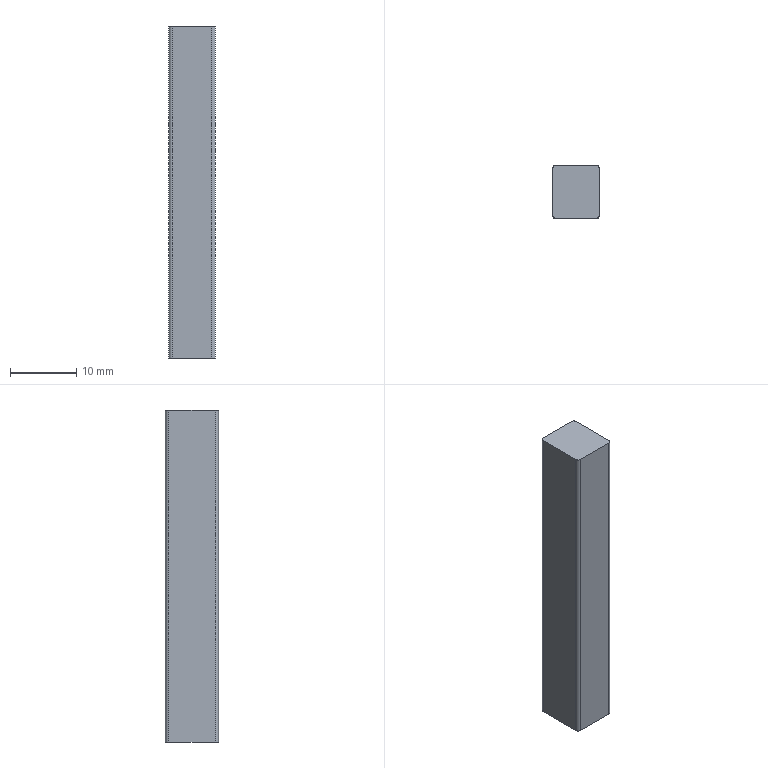Part | NX | features BREP 1 | 1 solid | 10 faces | box 7.02 x 8 x 50 mm | volume 2797 mm3 | plane 6 | cylinder 4 | commonest cylinder face diameters 1 x4
STEP:
#1=CARTESIAN_POINT('',(-3.01,4.,-40.6));
#2=VERTEX_POINT('',#1);
#3=CARTESIAN_POINT('',(-3.51,3.5,-40.6));
#4=VERTEX_POINT('',#3);
#5=CARTESIAN_POINT('',(-3.01,3.5,-40.6));
#6=DIRECTION('',(0.,0.,1.));
#7=DIRECTION('',(1.,0.,0.));
#8=AXIS2_PLACEMENT_3D('',#5,#6,#7);
#9=CIRCLE('',#8,0.5);
#10=EDGE_CURVE('',#2,#4,#9,.T.);
#11=ORIENTED_EDGE('',*,*,#10,.F.);
#12=CARTESIAN_POINT('',(-3.01,4.,-90.6));
#13=VERTEX_POINT('',#12);
#14=CARTESIAN_POINT('',(-3.01,4.,-90.6));
#15=DIRECTION('',(0.,0.,1.));
#16=VECTOR('',#15,1000.);
#17=LINE('',#14,#16);
#18=EDGE_CURVE('',#13,#2,#17,.T.);
#19=ORIENTED_EDGE('',*,*,#18,.F.);
#20=CARTESIAN_POINT('',(-3.51,3.5,-90.6));
#21=VERTEX_POINT('',#20);
#22=CARTESIAN_POINT('',(-3.01,3.5,-90.6));
#23=DIRECTION('',(0.,0.,1.));
#24=DIRECTION('',(1.,0.,0.));
#25=AXIS2_PLACEMENT_3D('',#22,#23,#24);
#26=CIRCLE('',#25,0.5);
#27=EDGE_CURVE('',#13,#21,#26,.T.);
#28=ORIENTED_EDGE('',*,*,#27,.T.);
#29=CARTESIAN_POINT('',(-3.51,3.5,-90.6));
#30=DIRECTION('',(0.,0.,1.));
#31=VECTOR('',#30,1000.);
#32=LINE('',#29,#31);
#33=EDGE_CURVE('',#21,#4,#32,.T.);
#34=ORIENTED_EDGE('',*,*,#33,.T.);
#35=EDGE_LOOP('',(#11,#19,#28,#34));
#36=FACE_BOUND('',#35,.T.);
#37=CARTESIAN_POINT('',(-3.01,3.5,-90.6));
#38=DIRECTION('',(0.,0.,1.));
#39=DIRECTION('',(-1.,0.,0.));
#40=AXIS2_PLACEMENT_3D('',#37,#38,#39);
#41=CYLINDRICAL_SURFACE('',#40,0.5);
#42=ADVANCED_FACE('',(#36),#41,.T.);
#43=CARTESIAN_POINT('',(-3.51,-3.5,-40.6));
#44=VERTEX_POINT('',#43);
#45=CARTESIAN_POINT('',(-3.51,-3.5,-40.6));
#46=DIRECTION('',(0.,1.,0.));
#47=VECTOR('',#46,1000.);
#48=LINE('',#45,#47);
#49=EDGE_CURVE('',#44,#4,#48,.T.);
#50=ORIENTED_EDGE('',*,*,#49,.T.);
#51=ORIENTED_EDGE('',*,*,#33,.F.);
#52=CARTESIAN_POINT('',(-3.51,-3.5,-90.6));
#53=VERTEX_POINT('',#52);
#54=CARTESIAN_POINT('',(-3.51,-3.5,-90.6));
#55=DIRECTION('',(0.,1.,0.));
#56=VECTOR('',#55,1000.);
#57=LINE('',#54,#56);
#58=EDGE_CURVE('',#53,#21,#57,.T.);
#59=ORIENTED_EDGE('',*,*,#58,.F.);
#60=CARTESIAN_POINT('',(-3.51,-3.5,-90.6));
#61=DIRECTION('',(0.,0.,1.));
#62=VECTOR('',#61,1000.);
#63=LINE('',#60,#62);
#64=EDGE_CURVE('',#53,#44,#63,.T.);
#65=ORIENTED_EDGE('',*,*,#64,.T.);
#66=EDGE_LOOP('',(#50,#51,#59,#65));
#67=FACE_BOUND('',#66,.T.);
#68=CARTESIAN_POINT('',(-3.51,-3.5,-90.6));
#69=DIRECTION('',(1.,0.,0.));
#70=DIRECTION('',(0.,0.,1.));
#71=AXIS2_PLACEMENT_3D('',#68,#69,#70);
#72=PLANE('',#71);
#73=ADVANCED_FACE('',(#67),#72,.F.);
#74=CARTESIAN_POINT('',(-3.01,-4.,-40.6));
#75=VERTEX_POINT('',#74);
#76=CARTESIAN_POINT('',(-3.01,-3.5,-40.6));
#77=DIRECTION('',(0.,0.,1.));
#78=DIRECTION('',(1.,0.,0.));
#79=AXIS2_PLACEMENT_3D('',#76,#77,#78);
#80=CIRCLE('',#79,0.5);
#81=EDGE_CURVE('',#44,#75,#80,.T.);
#82=ORIENTED_EDGE('',*,*,#81,.F.);
#83=ORIENTED_EDGE('',*,*,#64,.F.);
#84=CARTESIAN_POINT('',(-3.01,-4.,-90.6));
#85=VERTEX_POINT('',#84);
#86=CARTESIAN_POINT('',(-3.01,-3.5,-90.6));
#87=DIRECTION('',(0.,0.,1.));
#88=DIRECTION('',(1.,0.,0.));
#89=AXIS2_PLACEMENT_3D('',#86,#87,#88);
#90=CIRCLE('',#89,0.5);
#91=EDGE_CURVE('',#53,#85,#90,.T.);
#92=ORIENTED_EDGE('',*,*,#91,.T.);
#93=CARTESIAN_POINT('',(-3.01,-4.,-90.6));
#94=DIRECTION('',(0.,0.,1.));
#95=VECTOR('',#94,1000.);
#96=LINE('',#93,#95);
#97=EDGE_CURVE('',#85,#75,#96,.T.);
#98=ORIENTED_EDGE('',*,*,#97,.T.);
#99=EDGE_LOOP('',(#82,#83,#92,#98));
#100=FACE_BOUND('',#99,.T.);
#101=CARTESIAN_POINT('',(-3.01,-3.5,-90.6));
#102=DIRECTION('',(0.,0.,1.));
#103=DIRECTION('',(-1.,0.,0.));
#104=AXIS2_PLACEMENT_3D('',#101,#102,#103);
#105=CYLINDRICAL_SURFACE('',#104,0.5);
#106=ADVANCED_FACE('',(#100),#105,.T.);
#107=CARTESIAN_POINT('',(3.01,-4.,-40.6));
#108=VERTEX_POINT('',#107);
#109=CARTESIAN_POINT('',(3.01,-4.,-40.6));
#110=DIRECTION('',(-1.,0.,0.));
#111=VECTOR('',#110,1000.);
#112=LINE('',#109,#111);
#113=EDGE_CURVE('',#108,#75,#112,.T.);
#114=ORIENTED_EDGE('',*,*,#113,.T.);
#115=ORIENTED_EDGE('',*,*,#97,.F.);
#116=CARTESIAN_POINT('',(3.01,-4.,-90.6));
#117=VERTEX_POINT('',#116);
#118=CARTESIAN_POINT('',(3.01,-4.,-90.6));
#119=DIRECTION('',(-1.,0.,0.));
#120=VECTOR('',#119,1000.);
#121=LINE('',#118,#120);
#122=EDGE_CURVE('',#117,#85,#121,.T.);
#123=ORIENTED_EDGE('',*,*,#122,.F.);
#124=CARTESIAN_POINT('',(3.01,-4.,-90.6));
#125=DIRECTION('',(0.,0.,1.));
#126=VECTOR('',#125,1000.);
#127=LINE('',#124,#126);
#128=EDGE_CURVE('',#117,#108,#127,.T.);
#129=ORIENTED_EDGE('',*,*,#128,.T.);
#130=EDGE_LOOP('',(#114,#115,#123,#129));
#131=FACE_BOUND('',#130,.T.);
#132=CARTESIAN_POINT('',(3.01,-4.,-90.6));
#133=DIRECTION('',(0.,1.,0.));
#134=DIRECTION('',(0.,0.,-1.));
#135=AXIS2_PLACEMENT_3D('',#132,#133,#134);
#136=PLANE('',#135);
#137=ADVANCED_FACE('',(#131),#136,.F.);
#138=CARTESIAN_POINT('',(3.51,-3.5,-40.6));
#139=VERTEX_POINT('',#138);
#140=CARTESIAN_POINT('',(3.01,-3.5,-40.6));
#141=DIRECTION('',(0.,0.,1.));
#142=DIRECTION('',(1.,0.,0.));
#143=AXIS2_PLACEMENT_3D('',#140,#141,#142);
#144=CIRCLE('',#143,0.5);
#145=EDGE_CURVE('',#108,#139,#144,.T.);
#146=ORIENTED_EDGE('',*,*,#145,.F.);
#147=ORIENTED_EDGE('',*,*,#128,.F.);
#148=CARTESIAN_POINT('',(3.51,-3.5,-90.6));
#149=VERTEX_POINT('',#148);
#150=CARTESIAN_POINT('',(3.01,-3.5,-90.6));
#151=DIRECTION('',(0.,0.,1.));
#152=DIRECTION('',(1.,0.,0.));
#153=AXIS2_PLACEMENT_3D('',#150,#151,#152);
#154=CIRCLE('',#153,0.5);
#155=EDGE_CURVE('',#117,#149,#154,.T.);
#156=ORIENTED_EDGE('',*,*,#155,.T.);
#157=CARTESIAN_POINT('',(3.51,-3.5,-90.6));
#158=DIRECTION('',(0.,0.,1.));
#159=VECTOR('',#158,1000.);
#160=LINE('',#157,#159);
#161=EDGE_CURVE('',#149,#139,#160,.T.);
#162=ORIENTED_EDGE('',*,*,#161,.T.);
#163=EDGE_LOOP('',(#146,#147,#156,#162));
#164=FACE_BOUND('',#163,.T.);
#165=CARTESIAN_POINT('',(3.01,-3.5,-90.6));
#166=DIRECTION('',(0.,0.,1.));
#167=DIRECTION('',(-1.,0.,0.));
#168=AXIS2_PLACEMENT_3D('',#165,#166,#167);
#169=CYLINDRICAL_SURFACE('',#168,0.5);
#170=ADVANCED_FACE('',(#164),#169,.T.);
#171=CARTESIAN_POINT('',(3.51,3.5,-40.6));
#172=VERTEX_POINT('',#171);
#173=CARTESIAN_POINT('',(3.51,3.5,-40.6));
#174=DIRECTION('',(0.,-1.,0.));
#175=VECTOR('',#174,1000.);
#176=LINE('',#173,#175);
#177=EDGE_CURVE('',#172,#139,#176,.T.);
#178=ORIENTED_EDGE('',*,*,#177,.T.);
#179=ORIENTED_EDGE('',*,*,#161,.F.);
#180=CARTESIAN_POINT('',(3.51,3.5,-90.6));
#181=VERTEX_POINT('',#180);
#182=CARTESIAN_POINT('',(3.51,3.5,-90.6));
#183=DIRECTION('',(0.,-1.,0.));
#184=VECTOR('',#183,1000.);
#185=LINE('',#182,#184);
#186=EDGE_CURVE('',#181,#149,#185,.T.);
#187=ORIENTED_EDGE('',*,*,#186,.F.);
#188=CARTESIAN_POINT('',(3.51,3.5,-90.6));
#189=DIRECTION('',(0.,0.,1.));
#190=VECTOR('',#189,1000.);
#191=LINE('',#188,#190);
#192=EDGE_CURVE('',#181,#172,#191,.T.);
#193=ORIENTED_EDGE('',*,*,#192,.T.);
#194=EDGE_LOOP('',(#178,#179,#187,#193));
#195=FACE_BOUND('',#194,.T.);
#196=CARTESIAN_POINT('',(3.51,3.5,-90.6));
#197=DIRECTION('',(-1.,0.,0.));
#198=DIRECTION('',(0.,0.,-1.));
#199=AXIS2_PLACEMENT_3D('',#196,#197,#198);
#200=PLANE('',#199);
#201=ADVANCED_FACE('',(#195),#200,.F.);
#202=CARTESIAN_POINT('',(3.01,4.,-40.6));
#203=VERTEX_POINT('',#202);
#204=CARTESIAN_POINT('',(3.01,3.5,-40.6));
#205=DIRECTION('',(0.,0.,1.));
#206=DIRECTION('',(1.,0.,0.));
#207=AXIS2_PLACEMENT_3D('',#204,#205,#206);
#208=CIRCLE('',#207,0.5);
#209=EDGE_CURVE('',#172,#203,#208,.T.);
#210=ORIENTED_EDGE('',*,*,#209,.F.);
#211=ORIENTED_EDGE('',*,*,#192,.F.);
#212=CARTESIAN_POINT('',(3.01,4.,-90.6));
#213=VERTEX_POINT('',#212);
#214=CARTESIAN_POINT('',(3.01,3.5,-90.6));
#215=DIRECTION('',(0.,0.,1.));
#216=DIRECTION('',(1.,0.,0.));
#217=AXIS2_PLACEMENT_3D('',#214,#215,#216);
#218=CIRCLE('',#217,0.5);
#219=EDGE_CURVE('',#181,#213,#218,.T.);
#220=ORIENTED_EDGE('',*,*,#219,.T.);
#221=CARTESIAN_POINT('',(3.01,4.,-90.6));
#222=DIRECTION('',(0.,0.,1.));
#223=VECTOR('',#222,1000.);
#224=LINE('',#221,#223);
#225=EDGE_CURVE('',#213,#203,#224,.T.);
#226=ORIENTED_EDGE('',*,*,#225,.T.);
#227=EDGE_LOOP('',(#210,#211,#220,#226));
#228=FACE_BOUND('',#227,.T.);
#229=CARTESIAN_POINT('',(3.01,3.5,-90.6));
#230=DIRECTION('',(0.,0.,1.));
#231=DIRECTION('',(-1.,0.,0.));
#232=AXIS2_PLACEMENT_3D('',#229,#230,#231);
#233=CYLINDRICAL_SURFACE('',#232,0.5);
#234=ADVANCED_FACE('',(#228),#233,.T.);
#235=CARTESIAN_POINT('',(-3.01,4.,-40.6));
#236=DIRECTION('',(1.,0.,0.));
#237=VECTOR('',#236,1000.);
#238=LINE('',#235,#237);
#239=EDGE_CURVE('',#2,#203,#238,.T.);
#240=ORIENTED_EDGE('',*,*,#239,.T.);
#241=ORIENTED_EDGE('',*,*,#225,.F.);
#242=CARTESIAN_POINT('',(-3.01,4.,-90.6));
#243=DIRECTION('',(1.,0.,0.));
#244=VECTOR('',#243,1000.);
#245=LINE('',#242,#244);
#246=EDGE_CURVE('',#13,#213,#245,.T.);
#247=ORIENTED_EDGE('',*,*,#246,.F.);
#248=ORIENTED_EDGE('',*,*,#18,.T.);
#249=EDGE_LOOP('',(#240,#241,#247,#248));
#250=FACE_BOUND('',#249,.T.);
#251=CARTESIAN_POINT('',(-3.01,4.,-90.6));
#252=DIRECTION('',(0.,-1.,0.));
#253=DIRECTION('',(0.,0.,1.));
#254=AXIS2_PLACEMENT_3D('',#251,#252,#253);
#255=PLANE('',#254);
#256=ADVANCED_FACE('',(#250),#255,.F.);
#257=ORIENTED_EDGE('',*,*,#27,.F.);
#258=ORIENTED_EDGE('',*,*,#246,.T.);
#259=ORIENTED_EDGE('',*,*,#219,.F.);
#260=ORIENTED_EDGE('',*,*,#186,.T.);
#261=ORIENTED_EDGE('',*,*,#155,.F.);
#262=ORIENTED_EDGE('',*,*,#122,.T.);
#263=ORIENTED_EDGE('',*,*,#91,.F.);
#264=ORIENTED_EDGE('',*,*,#58,.T.);
#265=EDGE_LOOP('',(#257,#258,#259,#260,#261,#262,#263,#264));
#266=FACE_BOUND('',#265,.T.);
#267=CARTESIAN_POINT('',(-3.01,3.5,-90.6));
#268=DIRECTION('',(0.,0.,1.));
#269=DIRECTION('',(-1.,0.,0.));
#270=AXIS2_PLACEMENT_3D('',#267,#268,#269);
#271=PLANE('',#270);
#272=ADVANCED_FACE('',(#266),#271,.F.);
#273=ORIENTED_EDGE('',*,*,#10,.T.);
#274=ORIENTED_EDGE('',*,*,#49,.F.);
#275=ORIENTED_EDGE('',*,*,#81,.T.);
#276=ORIENTED_EDGE('',*,*,#113,.F.);
#277=ORIENTED_EDGE('',*,*,#145,.T.);
#278=ORIENTED_EDGE('',*,*,#177,.F.);
#279=ORIENTED_EDGE('',*,*,#209,.T.);
#280=ORIENTED_EDGE('',*,*,#239,.F.);
#281=EDGE_LOOP('',(#273,#274,#275,#276,#277,#278,#279,#280));
#282=FACE_BOUND('',#281,.T.);
#283=CARTESIAN_POINT('',(-3.01,3.5,-40.6));
#284=DIRECTION('',(0.,0.,1.));
#285=DIRECTION('',(-1.,0.,0.));
#286=AXIS2_PLACEMENT_3D('',#283,#284,#285);
#287=PLANE('',#286);
#288=ADVANCED_FACE('',(#282),#287,.T.);
#289=CLOSED_SHELL('',(#42,#73,#106,#137,#170,#201,#234,#256,#272,#288));
#290=MANIFOLD_SOLID_BREP('',#289);
#291=(LENGTH_UNIT()NAMED_UNIT(*)SI_UNIT(.MILLI.,.METRE.));
#292=UNCERTAINTY_MEASURE_WITH_UNIT(LENGTH_MEASURE(0.00001),#291,'','');
#293=(NAMED_UNIT(*)PLANE_ANGLE_UNIT()SI_UNIT($,.RADIAN.));
#294=(NAMED_UNIT(*)SI_UNIT($,.STERADIAN.)SOLID_ANGLE_UNIT());
#295=(GEOMETRIC_REPRESENTATION_CONTEXT(3)GLOBAL_UNCERTAINTY_ASSIGNED_CONTEXT((#292))GLOBAL_UNIT_ASSIGNED_CONTEXT((#291,#293,#294))REPRESENTATION_CONTEXT('',''));
#296=ADVANCED_BREP_SHAPE_REPRESENTATION('',(#290),#295);